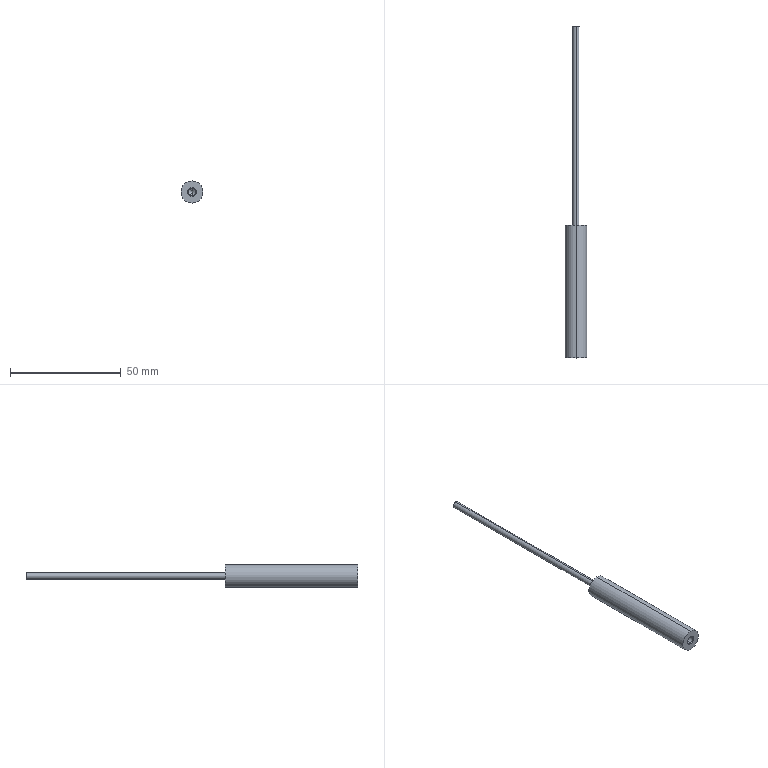Part | SolidWorks | features Extrusion 1, HoleWzd 1, ICE 1 | 1 solid | 13 faces | box 10 x 150 x 10 mm | volume 5247 mm3 | cylinder 6 | cone 4 | plane 3 | commonest cylinder face diameters 3 x2 3.3 x2 10 x2
STEP:
#1=CARTESIAN_POINT('',(0.,0.375,1.65));
#2=VERTEX_POINT('',#1);
#3=CARTESIAN_POINT('',(0.,0.375,-1.65));
#4=VERTEX_POINT('',#3);
#5=CARTESIAN_POINT('',(0.,0.375,0.));
#6=DIRECTION('',(0.,-1.,0.));
#7=DIRECTION('',(0.,0.,-1.));
#8=AXIS2_PLACEMENT_3D('',#5,#6,#7);
#9=CIRCLE('',#8,1.65);
#10=EDGE_CURVE('',#2,#4,#9,.T.);
#11=ORIENTED_EDGE('',*,*,#10,.F.);
#12=CARTESIAN_POINT('',(0.,0.,2.025));
#13=VERTEX_POINT('',#12);
#14=CARTESIAN_POINT('',(0.,0.,2.025));
#15=DIRECTION('',(0.,-0.7071,0.7071));
#16=VECTOR('',#15,1000.);
#17=LINE('',#14,#16);
#18=EDGE_CURVE('',#2,#13,#17,.T.);
#19=ORIENTED_EDGE('',*,*,#18,.T.);
#20=CARTESIAN_POINT('',(0.,0.,-2.025));
#21=VERTEX_POINT('',#20);
#22=CARTESIAN_POINT('',(0.,0.,0.));
#23=DIRECTION('',(0.,-1.,0.));
#24=DIRECTION('',(0.,0.,-1.));
#25=AXIS2_PLACEMENT_3D('',#22,#23,#24);
#26=CIRCLE('',#25,2.025);
#27=EDGE_CURVE('',#13,#21,#26,.T.);
#28=ORIENTED_EDGE('',*,*,#27,.T.);
#29=CARTESIAN_POINT('',(0.,0.,-2.025));
#30=DIRECTION('',(0.,-0.7071,-0.7071));
#31=VECTOR('',#30,1000.);
#32=LINE('',#29,#31);
#33=EDGE_CURVE('',#4,#21,#32,.T.);
#34=ORIENTED_EDGE('',*,*,#33,.F.);
#35=EDGE_LOOP('',(#11,#19,#28,#34));
#36=FACE_OUTER_BOUND('',#35,.T.);
#37=CARTESIAN_POINT('',(0.,0.,0.));
#38=DIRECTION('',(0.,-1.,0.));
#39=DIRECTION('',(0.,0.,-1.));
#40=AXIS2_PLACEMENT_3D('',#37,#38,#39);
#41=CONICAL_SURFACE('',#40,2.025,0.7854);
#42=ADVANCED_FACE('',(#36),#41,.F.);
#43=CARTESIAN_POINT('',(0.,11.5,1.65));
#44=VERTEX_POINT('',#43);
#45=CARTESIAN_POINT('',(0.,11.5,-1.65));
#46=VERTEX_POINT('',#45);
#47=CARTESIAN_POINT('',(0.,11.5,0.));
#48=DIRECTION('',(0.,-1.,0.));
#49=DIRECTION('',(0.,0.,-1.));
#50=AXIS2_PLACEMENT_3D('',#47,#48,#49);
#51=CIRCLE('',#50,1.65);
#52=EDGE_CURVE('',#44,#46,#51,.T.);
#53=ORIENTED_EDGE('',*,*,#52,.F.);
#54=CARTESIAN_POINT('',(0.,0.,1.65));
#55=DIRECTION('',(0.,-1.,0.));
#56=VECTOR('',#55,1000.);
#57=LINE('',#54,#56);
#58=EDGE_CURVE('',#44,#2,#57,.T.);
#59=ORIENTED_EDGE('',*,*,#58,.T.);
#60=ORIENTED_EDGE('',*,*,#10,.T.);
#61=CARTESIAN_POINT('',(0.,0.,-1.65));
#62=DIRECTION('',(0.,-1.,0.));
#63=VECTOR('',#62,1000.);
#64=LINE('',#61,#63);
#65=EDGE_CURVE('',#46,#4,#64,.T.);
#66=ORIENTED_EDGE('',*,*,#65,.F.);
#67=EDGE_LOOP('',(#53,#59,#60,#66));
#68=FACE_OUTER_BOUND('',#67,.T.);
#69=CARTESIAN_POINT('',(0.,0.,0.));
#70=DIRECTION('',(0.,-1.,0.));
#71=DIRECTION('',(0.,0.,-1.));
#72=AXIS2_PLACEMENT_3D('',#69,#70,#71);
#73=CYLINDRICAL_SURFACE('',#72,1.65);
#74=ADVANCED_FACE('',(#68),#73,.F.);
#75=CARTESIAN_POINT('',(0.,12.491,0.));
#76=VERTEX_POINT('',#75);
#77=CARTESIAN_POINT('',(0.,11.5,-1.65));
#78=DIRECTION('',(0.,-0.515,-0.8572));
#79=VECTOR('',#78,1000.);
#80=LINE('',#77,#79);
#81=EDGE_CURVE('',#76,#46,#80,.T.);
#82=ORIENTED_EDGE('',*,*,#81,.F.);
#83=CARTESIAN_POINT('',(0.,11.5,1.65));
#84=DIRECTION('',(0.,-0.515,0.8572));
#85=VECTOR('',#84,1000.);
#86=LINE('',#83,#85);
#87=EDGE_CURVE('',#76,#44,#86,.T.);
#88=ORIENTED_EDGE('',*,*,#87,.T.);
#89=ORIENTED_EDGE('',*,*,#52,.T.);
#90=EDGE_LOOP('',(#82,#88,#89));
#91=FACE_OUTER_BOUND('',#90,.T.);
#92=CARTESIAN_POINT('',(0.,11.5,0.));
#93=DIRECTION('',(0.,-1.,0.));
#94=DIRECTION('',(0.,0.,-1.));
#95=AXIS2_PLACEMENT_3D('',#92,#93,#94);
#96=CONICAL_SURFACE('',#95,1.65,1.03);
#97=ADVANCED_FACE('',(#91),#96,.F.);
#98=CARTESIAN_POINT('',(0.,150.,1.5));
#99=VERTEX_POINT('',#98);
#100=CARTESIAN_POINT('',(0.,150.,-1.5));
#101=VERTEX_POINT('',#100);
#102=CARTESIAN_POINT('',(0.,150.,0.));
#103=DIRECTION('',(0.,1.,0.));
#104=DIRECTION('',(0.,0.,1.));
#105=AXIS2_PLACEMENT_3D('',#102,#103,#104);
#106=CIRCLE('',#105,1.5);
#107=EDGE_CURVE('',#99,#101,#106,.T.);
#108=ORIENTED_EDGE('',*,*,#107,.F.);
#109=CARTESIAN_POINT('',(0.,60.,1.5));
#110=VERTEX_POINT('',#109);
#111=CARTESIAN_POINT('',(0.,150.,1.5));
#112=DIRECTION('',(0.,-1.,0.));
#113=VECTOR('',#112,1000.);
#114=LINE('',#111,#113);
#115=EDGE_CURVE('',#99,#110,#114,.T.);
#116=ORIENTED_EDGE('',*,*,#115,.T.);
#117=CARTESIAN_POINT('',(0.,60.,-1.5));
#118=VERTEX_POINT('',#117);
#119=CARTESIAN_POINT('',(0.,60.,0.));
#120=DIRECTION('',(0.,1.,0.));
#121=DIRECTION('',(0.,0.,1.));
#122=AXIS2_PLACEMENT_3D('',#119,#120,#121);
#123=CIRCLE('',#122,1.5);
#124=EDGE_CURVE('',#110,#118,#123,.T.);
#125=ORIENTED_EDGE('',*,*,#124,.T.);
#126=CARTESIAN_POINT('',(0.,150.,-1.5));
#127=DIRECTION('',(0.,-1.,0.));
#128=VECTOR('',#127,1000.);
#129=LINE('',#126,#128);
#130=EDGE_CURVE('',#101,#118,#129,.T.);
#131=ORIENTED_EDGE('',*,*,#130,.F.);
#132=EDGE_LOOP('',(#108,#116,#125,#131));
#133=FACE_OUTER_BOUND('',#132,.T.);
#134=CARTESIAN_POINT('',(0.,150.,0.));
#135=DIRECTION('',(0.,-1.,0.));
#136=DIRECTION('',(0.,0.,-1.));
#137=AXIS2_PLACEMENT_3D('',#134,#135,#136);
#138=CYLINDRICAL_SURFACE('',#137,1.5);
#139=ADVANCED_FACE('',(#133),#138,.T.);
#140=CARTESIAN_POINT('',(0.,60.,5.));
#141=VERTEX_POINT('',#140);
#142=CARTESIAN_POINT('',(0.,60.,-5.));
#143=VERTEX_POINT('',#142);
#144=CARTESIAN_POINT('',(0.,60.,0.));
#145=DIRECTION('',(0.,1.,0.));
#146=DIRECTION('',(0.,0.,1.));
#147=AXIS2_PLACEMENT_3D('',#144,#145,#146);
#148=CIRCLE('',#147,5.);
#149=EDGE_CURVE('',#141,#143,#148,.T.);
#150=ORIENTED_EDGE('',*,*,#149,.F.);
#151=CARTESIAN_POINT('',(0.,0.,5.));
#152=VERTEX_POINT('',#151);
#153=CARTESIAN_POINT('',(0.,60.,5.));
#154=DIRECTION('',(0.,-1.,0.));
#155=VECTOR('',#154,1000.);
#156=LINE('',#153,#155);
#157=EDGE_CURVE('',#141,#152,#156,.T.);
#158=ORIENTED_EDGE('',*,*,#157,.T.);
#159=CARTESIAN_POINT('',(0.,0.,-5.));
#160=VERTEX_POINT('',#159);
#161=CARTESIAN_POINT('',(0.,0.,0.));
#162=DIRECTION('',(0.,1.,0.));
#163=DIRECTION('',(0.,0.,1.));
#164=AXIS2_PLACEMENT_3D('',#161,#162,#163);
#165=CIRCLE('',#164,5.);
#166=EDGE_CURVE('',#152,#160,#165,.T.);
#167=ORIENTED_EDGE('',*,*,#166,.T.);
#168=CARTESIAN_POINT('',(0.,60.,-5.));
#169=DIRECTION('',(0.,-1.,0.));
#170=VECTOR('',#169,1000.);
#171=LINE('',#168,#170);
#172=EDGE_CURVE('',#143,#160,#171,.T.);
#173=ORIENTED_EDGE('',*,*,#172,.F.);
#174=EDGE_LOOP('',(#150,#158,#167,#173));
#175=FACE_OUTER_BOUND('',#174,.T.);
#176=CARTESIAN_POINT('',(0.,60.,0.));
#177=DIRECTION('',(0.,-1.,0.));
#178=DIRECTION('',(0.,0.,-1.));
#179=AXIS2_PLACEMENT_3D('',#176,#177,#178);
#180=CYLINDRICAL_SURFACE('',#179,5.);
#181=ADVANCED_FACE('',(#175),#180,.T.);
#182=ORIENTED_EDGE('',*,*,#157,.F.);
#183=CARTESIAN_POINT('',(0.,60.,0.));
#184=DIRECTION('',(0.,1.,0.));
#185=DIRECTION('',(0.,0.,1.));
#186=AXIS2_PLACEMENT_3D('',#183,#184,#185);
#187=CIRCLE('',#186,5.);
#188=EDGE_CURVE('',#143,#141,#187,.T.);
#189=ORIENTED_EDGE('',*,*,#188,.F.);
#190=ORIENTED_EDGE('',*,*,#172,.T.);
#191=CARTESIAN_POINT('',(0.,0.,0.));
#192=DIRECTION('',(0.,1.,0.));
#193=DIRECTION('',(0.,0.,1.));
#194=AXIS2_PLACEMENT_3D('',#191,#192,#193);
#195=CIRCLE('',#194,5.);
#196=EDGE_CURVE('',#160,#152,#195,.T.);
#197=ORIENTED_EDGE('',*,*,#196,.T.);
#198=EDGE_LOOP('',(#182,#189,#190,#197));
#199=FACE_OUTER_BOUND('',#198,.T.);
#200=CARTESIAN_POINT('',(0.,60.,0.));
#201=DIRECTION('',(0.,-1.,0.));
#202=DIRECTION('',(0.,0.,-1.));
#203=AXIS2_PLACEMENT_3D('',#200,#201,#202);
#204=CYLINDRICAL_SURFACE('',#203,5.);
#205=ADVANCED_FACE('',(#199),#204,.T.);
#206=CARTESIAN_POINT('',(0.,60.,0.));
#207=DIRECTION('',(0.,1.,0.));
#208=DIRECTION('',(0.,0.,1.));
#209=AXIS2_PLACEMENT_3D('',#206,#207,#208);
#210=CIRCLE('',#209,1.5);
#211=EDGE_CURVE('',#118,#110,#210,.T.);
#212=ORIENTED_EDGE('',*,*,#211,.F.);
#213=ORIENTED_EDGE('',*,*,#124,.F.);
#214=EDGE_LOOP('',(#212,#213));
#215=FACE_BOUND('',#214,.T.);
#216=ORIENTED_EDGE('',*,*,#188,.T.);
#217=ORIENTED_EDGE('',*,*,#149,.T.);
#218=EDGE_LOOP('',(#216,#217));
#219=FACE_OUTER_BOUND('',#218,.T.);
#220=CARTESIAN_POINT('',(0.,60.,0.));
#221=DIRECTION('',(0.,1.,0.));
#222=DIRECTION('',(0.,0.,1.));
#223=AXIS2_PLACEMENT_3D('',#220,#221,#222);
#224=PLANE('',#223);
#225=ADVANCED_FACE('',(#215,#219),#224,.T.);
#226=CARTESIAN_POINT('',(0.,0.,0.));
#227=DIRECTION('',(0.,-1.,0.));
#228=DIRECTION('',(0.,0.,-1.));
#229=AXIS2_PLACEMENT_3D('',#226,#227,#228);
#230=CIRCLE('',#229,2.025);
#231=EDGE_CURVE('',#21,#13,#230,.T.);
#232=ORIENTED_EDGE('',*,*,#231,.F.);
#233=ORIENTED_EDGE('',*,*,#27,.F.);
#234=EDGE_LOOP('',(#232,#233));
#235=FACE_BOUND('',#234,.T.);
#236=ORIENTED_EDGE('',*,*,#196,.F.);
#237=ORIENTED_EDGE('',*,*,#166,.F.);
#238=EDGE_LOOP('',(#236,#237));
#239=FACE_OUTER_BOUND('',#238,.T.);
#240=CARTESIAN_POINT('',(0.,0.,0.));
#241=DIRECTION('',(0.,1.,0.));
#242=DIRECTION('',(0.,0.,1.));
#243=AXIS2_PLACEMENT_3D('',#240,#241,#242);
#244=PLANE('',#243);
#245=ADVANCED_FACE('',(#235,#239),#244,.F.);
#246=ORIENTED_EDGE('',*,*,#115,.F.);
#247=CARTESIAN_POINT('',(0.,150.,0.));
#248=DIRECTION('',(0.,1.,0.));
#249=DIRECTION('',(0.,0.,1.));
#250=AXIS2_PLACEMENT_3D('',#247,#248,#249);
#251=CIRCLE('',#250,1.5);
#252=EDGE_CURVE('',#101,#99,#251,.T.);
#253=ORIENTED_EDGE('',*,*,#252,.F.);
#254=ORIENTED_EDGE('',*,*,#130,.T.);
#255=ORIENTED_EDGE('',*,*,#211,.T.);
#256=EDGE_LOOP('',(#246,#253,#254,#255));
#257=FACE_OUTER_BOUND('',#256,.T.);
#258=CARTESIAN_POINT('',(0.,150.,0.));
#259=DIRECTION('',(0.,-1.,0.));
#260=DIRECTION('',(0.,0.,-1.));
#261=AXIS2_PLACEMENT_3D('',#258,#259,#260);
#262=CYLINDRICAL_SURFACE('',#261,1.5);
#263=ADVANCED_FACE('',(#257),#262,.T.);
#264=ORIENTED_EDGE('',*,*,#252,.T.);
#265=ORIENTED_EDGE('',*,*,#107,.T.);
#266=EDGE_LOOP('',(#264,#265));
#267=FACE_OUTER_BOUND('',#266,.T.);
#268=CARTESIAN_POINT('',(0.,150.,0.));
#269=DIRECTION('',(0.,1.,0.));
#270=DIRECTION('',(0.,0.,1.));
#271=AXIS2_PLACEMENT_3D('',#268,#269,#270);
#272=PLANE('',#271);
#273=ADVANCED_FACE('',(#267),#272,.T.);
#274=ORIENTED_EDGE('',*,*,#87,.F.);
#275=ORIENTED_EDGE('',*,*,#81,.T.);
#276=CARTESIAN_POINT('',(0.,11.5,0.));
#277=DIRECTION('',(0.,-1.,0.));
#278=DIRECTION('',(0.,0.,-1.));
#279=AXIS2_PLACEMENT_3D('',#276,#277,#278);
#280=CIRCLE('',#279,1.65);
#281=EDGE_CURVE('',#46,#44,#280,.T.);
#282=ORIENTED_EDGE('',*,*,#281,.T.);
#283=EDGE_LOOP('',(#274,#275,#282));
#284=FACE_OUTER_BOUND('',#283,.T.);
#285=CARTESIAN_POINT('',(0.,11.5,0.));
#286=DIRECTION('',(0.,-1.,0.));
#287=DIRECTION('',(0.,0.,-1.));
#288=AXIS2_PLACEMENT_3D('',#285,#286,#287);
#289=CONICAL_SURFACE('',#288,1.65,1.03);
#290=ADVANCED_FACE('',(#284),#289,.F.);
#291=ORIENTED_EDGE('',*,*,#58,.F.);
#292=ORIENTED_EDGE('',*,*,#281,.F.);
#293=ORIENTED_EDGE('',*,*,#65,.T.);
#294=CARTESIAN_POINT('',(0.,0.375,0.));
#295=DIRECTION('',(0.,-1.,0.));
#296=DIRECTION('',(0.,0.,-1.));
#297=AXIS2_PLACEMENT_3D('',#294,#295,#296);
#298=CIRCLE('',#297,1.65);
#299=EDGE_CURVE('',#4,#2,#298,.T.);
#300=ORIENTED_EDGE('',*,*,#299,.T.);
#301=EDGE_LOOP('',(#291,#292,#293,#300));
#302=FACE_OUTER_BOUND('',#301,.T.);
#303=CARTESIAN_POINT('',(0.,0.,0.));
#304=DIRECTION('',(0.,-1.,0.));
#305=DIRECTION('',(0.,0.,-1.));
#306=AXIS2_PLACEMENT_3D('',#303,#304,#305);
#307=CYLINDRICAL_SURFACE('',#306,1.65);
#308=ADVANCED_FACE('',(#302),#307,.F.);
#309=ORIENTED_EDGE('',*,*,#18,.F.);
#310=ORIENTED_EDGE('',*,*,#299,.F.);
#311=ORIENTED_EDGE('',*,*,#33,.T.);
#312=ORIENTED_EDGE('',*,*,#231,.T.);
#313=EDGE_LOOP('',(#309,#310,#311,#312));
#314=FACE_OUTER_BOUND('',#313,.T.);
#315=CARTESIAN_POINT('',(0.,0.,0.));
#316=DIRECTION('',(0.,-1.,0.));
#317=DIRECTION('',(0.,0.,-1.));
#318=AXIS2_PLACEMENT_3D('',#315,#316,#317);
#319=CONICAL_SURFACE('',#318,2.025,0.7854);
#320=ADVANCED_FACE('',(#314),#319,.F.);
#321=CLOSED_SHELL('',(#42,#74,#97,#139,#181,#205,#225,#245,#263,#273,#290,#308,#320));
#322=MANIFOLD_SOLID_BREP('',#321);
#323=CARTESIAN_POINT('',(0.,0.,0.));
#324=DIRECTION('',(0.,0.,1.));
#325=DIRECTION('',(1.,0.,0.));
#326=AXIS2_PLACEMENT_3D('',#323,#324,#325);
#327=(LENGTH_UNIT()NAMED_UNIT(*)SI_UNIT(.MILLI.,.METRE.));
#328=UNCERTAINTY_MEASURE_WITH_UNIT(LENGTH_MEASURE(0.00001),#327,'','');
#329=(NAMED_UNIT(*)PLANE_ANGLE_UNIT()SI_UNIT($,.RADIAN.));
#330=(NAMED_UNIT(*)SI_UNIT($,.STERADIAN.)SOLID_ANGLE_UNIT());
#331=(GEOMETRIC_REPRESENTATION_CONTEXT(3)GLOBAL_UNCERTAINTY_ASSIGNED_CONTEXT((#328))GLOBAL_UNIT_ASSIGNED_CONTEXT((#327,#329,#330))REPRESENTATION_CONTEXT('',''));
#332=ADVANCED_BREP_SHAPE_REPRESENTATION('',(#322,#326),#331);